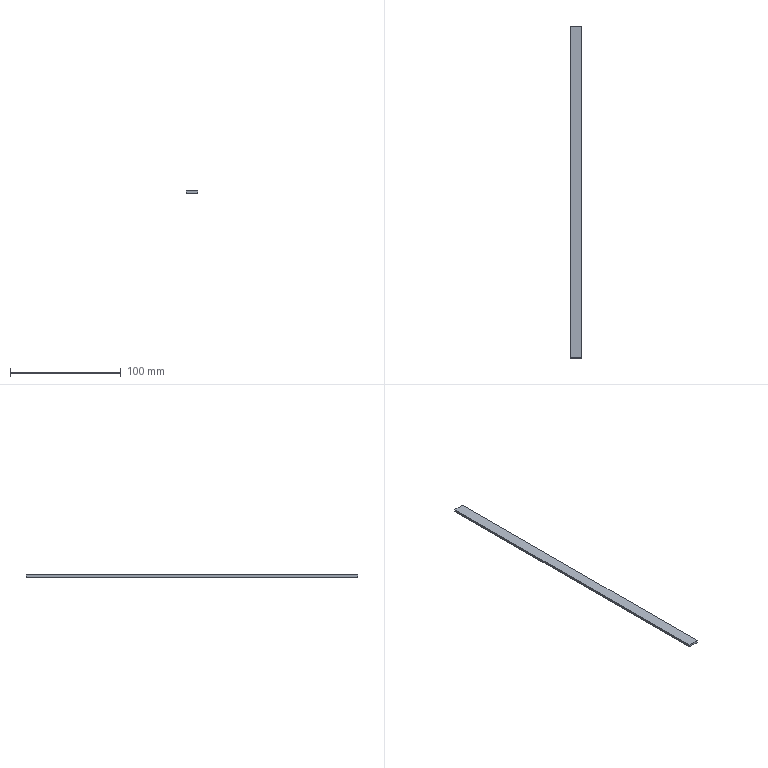Part | SolidWorks | features Extrusion 1 | 1 solid | 6 faces | box 10 x 300 x 2 mm | volume 6000 mm3 | plane 6
STEP:
#1=CARTESIAN_POINT('',(0.,300.,0.));
#2=VERTEX_POINT('',#1);
#3=CARTESIAN_POINT('',(0.,0.,0.));
#4=VERTEX_POINT('',#3);
#5=CARTESIAN_POINT('',(0.,0.,0.));
#6=DIRECTION('',(0.,-1.,0.));
#7=VECTOR('',#6,1000.);
#8=LINE('',#5,#7);
#9=EDGE_CURVE('',#2,#4,#8,.T.);
#10=ORIENTED_EDGE('',*,*,#9,.T.);
#11=CARTESIAN_POINT('',(0.,0.,2.));
#12=VERTEX_POINT('',#11);
#13=CARTESIAN_POINT('',(0.,0.,2.));
#14=DIRECTION('',(0.,0.,-1.));
#15=VECTOR('',#14,1000.);
#16=LINE('',#13,#15);
#17=EDGE_CURVE('',#12,#4,#16,.T.);
#18=ORIENTED_EDGE('',*,*,#17,.F.);
#19=CARTESIAN_POINT('',(0.,300.,2.));
#20=VERTEX_POINT('',#19);
#21=CARTESIAN_POINT('',(0.,0.,2.));
#22=DIRECTION('',(0.,-1.,0.));
#23=VECTOR('',#22,1000.);
#24=LINE('',#21,#23);
#25=EDGE_CURVE('',#20,#12,#24,.T.);
#26=ORIENTED_EDGE('',*,*,#25,.F.);
#27=CARTESIAN_POINT('',(0.,300.,2.));
#28=DIRECTION('',(0.,0.,-1.));
#29=VECTOR('',#28,1000.);
#30=LINE('',#27,#29);
#31=EDGE_CURVE('',#20,#2,#30,.T.);
#32=ORIENTED_EDGE('',*,*,#31,.T.);
#33=EDGE_LOOP('',(#10,#18,#26,#32));
#34=FACE_OUTER_BOUND('',#33,.T.);
#35=CARTESIAN_POINT('',(0.,0.,2.));
#36=DIRECTION('',(1.,0.,0.));
#37=DIRECTION('',(0.,0.,-1.));
#38=AXIS2_PLACEMENT_3D('',#35,#36,#37);
#39=PLANE('',#38);
#40=ADVANCED_FACE('',(#34),#39,.F.);
#41=CARTESIAN_POINT('',(10.,0.,0.));
#42=VERTEX_POINT('',#41);
#43=CARTESIAN_POINT('',(0.,0.,0.));
#44=DIRECTION('',(1.,0.,0.));
#45=VECTOR('',#44,1000.);
#46=LINE('',#43,#45);
#47=EDGE_CURVE('',#4,#42,#46,.T.);
#48=ORIENTED_EDGE('',*,*,#47,.T.);
#49=CARTESIAN_POINT('',(10.,0.,2.));
#50=VERTEX_POINT('',#49);
#51=CARTESIAN_POINT('',(10.,0.,2.));
#52=DIRECTION('',(0.,0.,-1.));
#53=VECTOR('',#52,1000.);
#54=LINE('',#51,#53);
#55=EDGE_CURVE('',#50,#42,#54,.T.);
#56=ORIENTED_EDGE('',*,*,#55,.F.);
#57=CARTESIAN_POINT('',(0.,0.,2.));
#58=DIRECTION('',(1.,0.,0.));
#59=VECTOR('',#58,1000.);
#60=LINE('',#57,#59);
#61=EDGE_CURVE('',#12,#50,#60,.T.);
#62=ORIENTED_EDGE('',*,*,#61,.F.);
#63=ORIENTED_EDGE('',*,*,#17,.T.);
#64=EDGE_LOOP('',(#48,#56,#62,#63));
#65=FACE_OUTER_BOUND('',#64,.T.);
#66=CARTESIAN_POINT('',(0.,0.,2.));
#67=DIRECTION('',(0.,1.,0.));
#68=DIRECTION('',(0.,0.,1.));
#69=AXIS2_PLACEMENT_3D('',#66,#67,#68);
#70=PLANE('',#69);
#71=ADVANCED_FACE('',(#65),#70,.F.);
#72=CARTESIAN_POINT('',(10.,300.,0.));
#73=VERTEX_POINT('',#72);
#74=CARTESIAN_POINT('',(10.,0.,0.));
#75=DIRECTION('',(0.,1.,0.));
#76=VECTOR('',#75,1000.);
#77=LINE('',#74,#76);
#78=EDGE_CURVE('',#42,#73,#77,.T.);
#79=ORIENTED_EDGE('',*,*,#78,.T.);
#80=CARTESIAN_POINT('',(10.,300.,2.));
#81=VERTEX_POINT('',#80);
#82=CARTESIAN_POINT('',(10.,300.,2.));
#83=DIRECTION('',(0.,0.,-1.));
#84=VECTOR('',#83,1000.);
#85=LINE('',#82,#84);
#86=EDGE_CURVE('',#81,#73,#85,.T.);
#87=ORIENTED_EDGE('',*,*,#86,.F.);
#88=CARTESIAN_POINT('',(10.,0.,2.));
#89=DIRECTION('',(0.,1.,0.));
#90=VECTOR('',#89,1000.);
#91=LINE('',#88,#90);
#92=EDGE_CURVE('',#50,#81,#91,.T.);
#93=ORIENTED_EDGE('',*,*,#92,.F.);
#94=ORIENTED_EDGE('',*,*,#55,.T.);
#95=EDGE_LOOP('',(#79,#87,#93,#94));
#96=FACE_OUTER_BOUND('',#95,.T.);
#97=CARTESIAN_POINT('',(10.,0.,2.));
#98=DIRECTION('',(-1.,0.,0.));
#99=DIRECTION('',(0.,0.,1.));
#100=AXIS2_PLACEMENT_3D('',#97,#98,#99);
#101=PLANE('',#100);
#102=ADVANCED_FACE('',(#96),#101,.F.);
#103=CARTESIAN_POINT('',(0.,300.,0.));
#104=DIRECTION('',(-1.,0.,0.));
#105=VECTOR('',#104,1000.);
#106=LINE('',#103,#105);
#107=EDGE_CURVE('',#73,#2,#106,.T.);
#108=ORIENTED_EDGE('',*,*,#107,.T.);
#109=ORIENTED_EDGE('',*,*,#31,.F.);
#110=CARTESIAN_POINT('',(0.,300.,2.));
#111=DIRECTION('',(-1.,0.,0.));
#112=VECTOR('',#111,1000.);
#113=LINE('',#110,#112);
#114=EDGE_CURVE('',#81,#20,#113,.T.);
#115=ORIENTED_EDGE('',*,*,#114,.F.);
#116=ORIENTED_EDGE('',*,*,#86,.T.);
#117=EDGE_LOOP('',(#108,#109,#115,#116));
#118=FACE_OUTER_BOUND('',#117,.T.);
#119=CARTESIAN_POINT('',(0.,300.,2.));
#120=DIRECTION('',(0.,-1.,0.));
#121=DIRECTION('',(0.,0.,-1.));
#122=AXIS2_PLACEMENT_3D('',#119,#120,#121);
#123=PLANE('',#122);
#124=ADVANCED_FACE('',(#118),#123,.F.);
#125=ORIENTED_EDGE('',*,*,#25,.T.);
#126=ORIENTED_EDGE('',*,*,#61,.T.);
#127=ORIENTED_EDGE('',*,*,#92,.T.);
#128=ORIENTED_EDGE('',*,*,#114,.T.);
#129=EDGE_LOOP('',(#125,#126,#127,#128));
#130=FACE_OUTER_BOUND('',#129,.T.);
#131=CARTESIAN_POINT('',(0.,0.,2.));
#132=DIRECTION('',(0.,0.,-1.));
#133=DIRECTION('',(-1.,0.,0.));
#134=AXIS2_PLACEMENT_3D('',#131,#132,#133);
#135=PLANE('',#134);
#136=ADVANCED_FACE('',(#130),#135,.F.);
#137=ORIENTED_EDGE('',*,*,#9,.F.);
#138=ORIENTED_EDGE('',*,*,#107,.F.);
#139=ORIENTED_EDGE('',*,*,#78,.F.);
#140=ORIENTED_EDGE('',*,*,#47,.F.);
#141=EDGE_LOOP('',(#137,#138,#139,#140));
#142=FACE_OUTER_BOUND('',#141,.T.);
#143=CARTESIAN_POINT('',(0.,0.,0.));
#144=DIRECTION('',(0.,0.,-1.));
#145=DIRECTION('',(-1.,0.,0.));
#146=AXIS2_PLACEMENT_3D('',#143,#144,#145);
#147=PLANE('',#146);
#148=ADVANCED_FACE('',(#142),#147,.T.);
#149=CLOSED_SHELL('',(#40,#71,#102,#124,#136,#148));
#150=MANIFOLD_SOLID_BREP('',#149);
#151=CARTESIAN_POINT('',(0.,0.,0.));
#152=DIRECTION('',(0.,0.,1.));
#153=DIRECTION('',(1.,0.,0.));
#154=AXIS2_PLACEMENT_3D('',#151,#152,#153);
#155=(LENGTH_UNIT()NAMED_UNIT(*)SI_UNIT(.MILLI.,.METRE.));
#156=UNCERTAINTY_MEASURE_WITH_UNIT(LENGTH_MEASURE(0.00001),#155,'','');
#157=(NAMED_UNIT(*)PLANE_ANGLE_UNIT()SI_UNIT($,.RADIAN.));
#158=(NAMED_UNIT(*)SI_UNIT($,.STERADIAN.)SOLID_ANGLE_UNIT());
#159=(GEOMETRIC_REPRESENTATION_CONTEXT(3)GLOBAL_UNCERTAINTY_ASSIGNED_CONTEXT((#156))GLOBAL_UNIT_ASSIGNED_CONTEXT((#155,#157,#158))REPRESENTATION_CONTEXT('',''));
#160=ADVANCED_BREP_SHAPE_REPRESENTATION('',(#150,#154),#159);